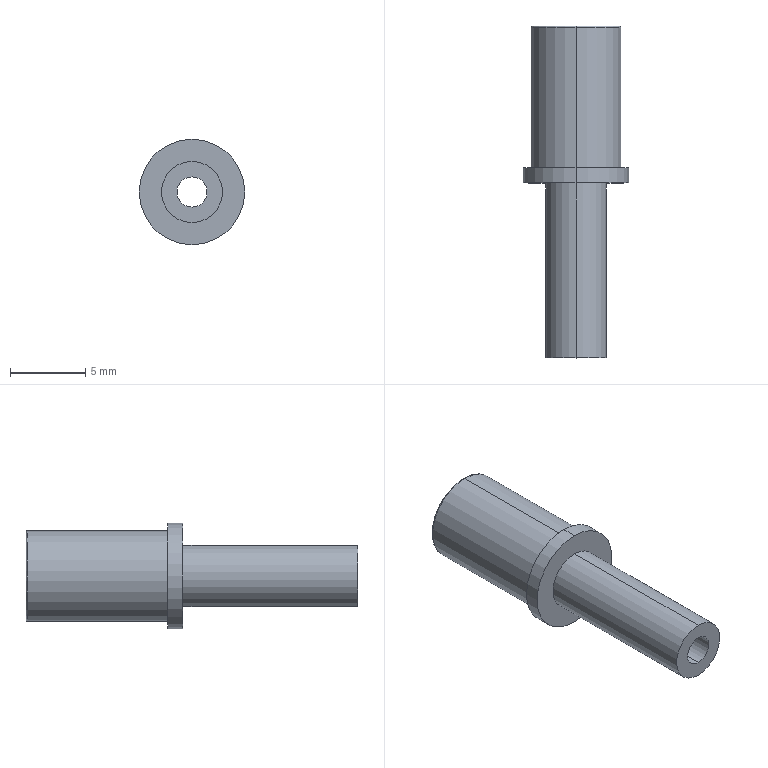Part | SolidWorks | features Fillet 1, Revolution 1 | 1 solid | 14 faces | box 7 x 22 x 7 mm | volume 384.292 mm3 | cylinder 8 | plane 4 | torus 2 | commonest cylinder face diameters 2 x2 4.047 x2 6 x2 7 x2
STEP:
#1=CARTESIAN_POINT('',(0.,10.4,2.9));
#2=VERTEX_POINT('',#1);
#3=CARTESIAN_POINT('',(0.,10.4,-2.9));
#4=VERTEX_POINT('',#3);
#5=CARTESIAN_POINT('',(0.,10.4,0.));
#6=DIRECTION('',(0.,1.,0.));
#7=DIRECTION('',(0.,0.,-1.));
#8=AXIS2_PLACEMENT_3D('',#5,#6,#7);
#9=CIRCLE('',#8,2.9);
#10=EDGE_CURVE('',#2,#4,#9,.T.);
#11=ORIENTED_EDGE('',*,*,#10,.F.);
#12=CARTESIAN_POINT('',(0.,10.3,3.));
#13=VERTEX_POINT('',#12);
#14=CARTESIAN_POINT('',(0.,10.3,2.9));
#15=DIRECTION('',(1.,0.,0.));
#16=DIRECTION('',(0.,0.,-1.));
#17=AXIS2_PLACEMENT_3D('',#14,#15,#16);
#18=CIRCLE('',#17,0.1);
#19=EDGE_CURVE('',#2,#13,#18,.T.);
#20=ORIENTED_EDGE('',*,*,#19,.T.);
#21=CARTESIAN_POINT('',(0.,10.3,-3.));
#22=VERTEX_POINT('',#21);
#23=CARTESIAN_POINT('',(0.,10.3,0.));
#24=DIRECTION('',(0.,-1.,0.));
#25=DIRECTION('',(0.,0.,-1.));
#26=AXIS2_PLACEMENT_3D('',#23,#24,#25);
#27=CIRCLE('',#26,3.);
#28=EDGE_CURVE('',#22,#13,#27,.T.);
#29=ORIENTED_EDGE('',*,*,#28,.F.);
#30=CARTESIAN_POINT('',(0.,10.3,-2.9));
#31=DIRECTION('',(-1.,0.,0.));
#32=DIRECTION('',(0.,0.,1.));
#33=AXIS2_PLACEMENT_3D('',#30,#31,#32);
#34=CIRCLE('',#33,0.1);
#35=EDGE_CURVE('',#4,#22,#34,.T.);
#36=ORIENTED_EDGE('',*,*,#35,.F.);
#37=EDGE_LOOP('',(#11,#20,#29,#36));
#38=FACE_OUTER_BOUND('',#37,.T.);
#39=CARTESIAN_POINT('',(0.,10.3,0.));
#40=DIRECTION('',(0.,-1.,0.));
#41=DIRECTION('',(0.,0.,-1.));
#42=AXIS2_PLACEMENT_3D('',#39,#40,#41);
#43=TOROIDAL_SURFACE('',#42,2.9,0.1);
#44=ADVANCED_FACE('',(#38),#43,.T.);
#45=CARTESIAN_POINT('',(0.,1.,-3.5));
#46=VERTEX_POINT('',#45);
#47=CARTESIAN_POINT('',(0.,1.,3.5));
#48=VERTEX_POINT('',#47);
#49=CARTESIAN_POINT('',(0.,1.,0.));
#50=DIRECTION('',(0.,-1.,0.));
#51=DIRECTION('',(0.,0.,-1.));
#52=AXIS2_PLACEMENT_3D('',#49,#50,#51);
#53=CIRCLE('',#52,3.5);
#54=EDGE_CURVE('',#46,#48,#53,.T.);
#55=ORIENTED_EDGE('',*,*,#54,.T.);
#56=CARTESIAN_POINT('',(0.,0.,3.5));
#57=VERTEX_POINT('',#56);
#58=CARTESIAN_POINT('',(0.,-19.747,3.5));
#59=DIRECTION('',(0.,-1.,0.));
#60=VECTOR('',#59,1000.);
#61=LINE('',#58,#60);
#62=EDGE_CURVE('',#48,#57,#61,.T.);
#63=ORIENTED_EDGE('',*,*,#62,.T.);
#64=CARTESIAN_POINT('',(0.,0.,-3.5));
#65=VERTEX_POINT('',#64);
#66=CARTESIAN_POINT('',(0.,0.,0.));
#67=DIRECTION('',(0.,-1.,0.));
#68=DIRECTION('',(0.,0.,-1.));
#69=AXIS2_PLACEMENT_3D('',#66,#67,#68);
#70=CIRCLE('',#69,3.5);
#71=EDGE_CURVE('',#65,#57,#70,.T.);
#72=ORIENTED_EDGE('',*,*,#71,.F.);
#73=CARTESIAN_POINT('',(0.,-19.747,-3.5));
#74=DIRECTION('',(0.,-1.,0.));
#75=VECTOR('',#74,1000.);
#76=LINE('',#73,#75);
#77=EDGE_CURVE('',#46,#65,#76,.T.);
#78=ORIENTED_EDGE('',*,*,#77,.F.);
#79=EDGE_LOOP('',(#55,#63,#72,#78));
#80=FACE_OUTER_BOUND('',#79,.T.);
#81=CARTESIAN_POINT('',(0.,-19.747,0.));
#82=DIRECTION('',(0.,-1.,0.));
#83=DIRECTION('',(0.,0.,-1.));
#84=AXIS2_PLACEMENT_3D('',#81,#82,#83);
#85=CYLINDRICAL_SURFACE('',#84,3.5);
#86=ADVANCED_FACE('',(#80),#85,.T.);
#87=CARTESIAN_POINT('',(0.,0.,-2.023));
#88=VERTEX_POINT('',#87);
#89=CARTESIAN_POINT('',(0.,0.,2.023));
#90=VERTEX_POINT('',#89);
#91=CARTESIAN_POINT('',(0.,0.,0.));
#92=DIRECTION('',(0.,-1.,0.));
#93=DIRECTION('',(0.,0.,-1.));
#94=AXIS2_PLACEMENT_3D('',#91,#92,#93);
#95=CIRCLE('',#94,2.023);
#96=EDGE_CURVE('',#88,#90,#95,.T.);
#97=ORIENTED_EDGE('',*,*,#96,.T.);
#98=CARTESIAN_POINT('',(0.,-11.6,2.023));
#99=VERTEX_POINT('',#98);
#100=CARTESIAN_POINT('',(0.,-19.747,2.023));
#101=DIRECTION('',(0.,-1.,0.));
#102=VECTOR('',#101,1000.);
#103=LINE('',#100,#102);
#104=EDGE_CURVE('',#90,#99,#103,.T.);
#105=ORIENTED_EDGE('',*,*,#104,.T.);
#106=CARTESIAN_POINT('',(0.,-11.6,-2.023));
#107=VERTEX_POINT('',#106);
#108=CARTESIAN_POINT('',(0.,-11.6,0.));
#109=DIRECTION('',(0.,-1.,0.));
#110=DIRECTION('',(0.,0.,-1.));
#111=AXIS2_PLACEMENT_3D('',#108,#109,#110);
#112=CIRCLE('',#111,2.023);
#113=EDGE_CURVE('',#107,#99,#112,.T.);
#114=ORIENTED_EDGE('',*,*,#113,.F.);
#115=CARTESIAN_POINT('',(0.,-19.747,-2.023));
#116=DIRECTION('',(0.,-1.,0.));
#117=VECTOR('',#116,1000.);
#118=LINE('',#115,#117);
#119=EDGE_CURVE('',#88,#107,#118,.T.);
#120=ORIENTED_EDGE('',*,*,#119,.F.);
#121=EDGE_LOOP('',(#97,#105,#114,#120));
#122=FACE_OUTER_BOUND('',#121,.T.);
#123=CARTESIAN_POINT('',(0.,-19.747,0.));
#124=DIRECTION('',(0.,-1.,0.));
#125=DIRECTION('',(0.,0.,-1.));
#126=AXIS2_PLACEMENT_3D('',#123,#124,#125);
#127=CYLINDRICAL_SURFACE('',#126,2.023);
#128=ADVANCED_FACE('',(#122),#127,.T.);
#129=CARTESIAN_POINT('',(0.,10.4,1.));
#130=VERTEX_POINT('',#129);
#131=CARTESIAN_POINT('',(0.,10.4,-1.));
#132=VERTEX_POINT('',#131);
#133=CARTESIAN_POINT('',(0.,10.4,0.));
#134=DIRECTION('',(0.,-1.,0.));
#135=DIRECTION('',(0.,0.,-1.));
#136=AXIS2_PLACEMENT_3D('',#133,#134,#135);
#137=CIRCLE('',#136,1.);
#138=EDGE_CURVE('',#130,#132,#137,.T.);
#139=ORIENTED_EDGE('',*,*,#138,.F.);
#140=CARTESIAN_POINT('',(0.,-11.6,1.));
#141=VERTEX_POINT('',#140);
#142=CARTESIAN_POINT('',(0.,-19.747,1.));
#143=DIRECTION('',(0.,-1.,0.));
#144=VECTOR('',#143,1000.);
#145=LINE('',#142,#144);
#146=EDGE_CURVE('',#130,#141,#145,.T.);
#147=ORIENTED_EDGE('',*,*,#146,.T.);
#148=CARTESIAN_POINT('',(0.,-11.6,-1.));
#149=VERTEX_POINT('',#148);
#150=CARTESIAN_POINT('',(0.,-11.6,0.));
#151=DIRECTION('',(0.,-1.,0.));
#152=DIRECTION('',(0.,0.,-1.));
#153=AXIS2_PLACEMENT_3D('',#150,#151,#152);
#154=CIRCLE('',#153,1.);
#155=EDGE_CURVE('',#141,#149,#154,.T.);
#156=ORIENTED_EDGE('',*,*,#155,.T.);
#157=CARTESIAN_POINT('',(0.,-19.747,-1.));
#158=DIRECTION('',(0.,-1.,0.));
#159=VECTOR('',#158,1000.);
#160=LINE('',#157,#159);
#161=EDGE_CURVE('',#132,#149,#160,.T.);
#162=ORIENTED_EDGE('',*,*,#161,.F.);
#163=EDGE_LOOP('',(#139,#147,#156,#162));
#164=FACE_OUTER_BOUND('',#163,.T.);
#165=CARTESIAN_POINT('',(0.,-19.747,0.));
#166=DIRECTION('',(0.,-1.,0.));
#167=DIRECTION('',(0.,0.,-1.));
#168=AXIS2_PLACEMENT_3D('',#165,#166,#167);
#169=CYLINDRICAL_SURFACE('',#168,1.);
#170=ADVANCED_FACE('',(#164),#169,.F.);
#171=ORIENTED_EDGE('',*,*,#28,.T.);
#172=CARTESIAN_POINT('',(0.,1.,3.));
#173=VERTEX_POINT('',#172);
#174=CARTESIAN_POINT('',(0.,-19.747,3.));
#175=DIRECTION('',(0.,-1.,0.));
#176=VECTOR('',#175,1000.);
#177=LINE('',#174,#176);
#178=EDGE_CURVE('',#13,#173,#177,.T.);
#179=ORIENTED_EDGE('',*,*,#178,.T.);
#180=CARTESIAN_POINT('',(0.,1.,-3.));
#181=VERTEX_POINT('',#180);
#182=CARTESIAN_POINT('',(0.,1.,0.));
#183=DIRECTION('',(0.,-1.,0.));
#184=DIRECTION('',(0.,0.,-1.));
#185=AXIS2_PLACEMENT_3D('',#182,#183,#184);
#186=CIRCLE('',#185,3.);
#187=EDGE_CURVE('',#181,#173,#186,.T.);
#188=ORIENTED_EDGE('',*,*,#187,.F.);
#189=CARTESIAN_POINT('',(0.,-19.747,-3.));
#190=DIRECTION('',(0.,-1.,0.));
#191=VECTOR('',#190,1000.);
#192=LINE('',#189,#191);
#193=EDGE_CURVE('',#22,#181,#192,.T.);
#194=ORIENTED_EDGE('',*,*,#193,.F.);
#195=EDGE_LOOP('',(#171,#179,#188,#194));
#196=FACE_OUTER_BOUND('',#195,.T.);
#197=CARTESIAN_POINT('',(0.,-19.747,0.));
#198=DIRECTION('',(0.,-1.,0.));
#199=DIRECTION('',(0.,0.,-1.));
#200=AXIS2_PLACEMENT_3D('',#197,#198,#199);
#201=CYLINDRICAL_SURFACE('',#200,3.);
#202=ADVANCED_FACE('',(#196),#201,.T.);
#203=ORIENTED_EDGE('',*,*,#178,.F.);
#204=CARTESIAN_POINT('',(0.,10.3,0.));
#205=DIRECTION('',(0.,-1.,0.));
#206=DIRECTION('',(0.,0.,-1.));
#207=AXIS2_PLACEMENT_3D('',#204,#205,#206);
#208=CIRCLE('',#207,3.);
#209=EDGE_CURVE('',#13,#22,#208,.T.);
#210=ORIENTED_EDGE('',*,*,#209,.T.);
#211=ORIENTED_EDGE('',*,*,#193,.T.);
#212=CARTESIAN_POINT('',(0.,1.,0.));
#213=DIRECTION('',(0.,-1.,0.));
#214=DIRECTION('',(0.,0.,-1.));
#215=AXIS2_PLACEMENT_3D('',#212,#213,#214);
#216=CIRCLE('',#215,3.);
#217=EDGE_CURVE('',#173,#181,#216,.T.);
#218=ORIENTED_EDGE('',*,*,#217,.F.);
#219=EDGE_LOOP('',(#203,#210,#211,#218));
#220=FACE_OUTER_BOUND('',#219,.T.);
#221=CARTESIAN_POINT('',(0.,-19.747,0.));
#222=DIRECTION('',(0.,-1.,0.));
#223=DIRECTION('',(0.,0.,-1.));
#224=AXIS2_PLACEMENT_3D('',#221,#222,#223);
#225=CYLINDRICAL_SURFACE('',#224,3.);
#226=ADVANCED_FACE('',(#220),#225,.T.);
#227=CARTESIAN_POINT('',(0.,10.4,0.));
#228=DIRECTION('',(0.,1.,0.));
#229=DIRECTION('',(0.,0.,-1.));
#230=AXIS2_PLACEMENT_3D('',#227,#228,#229);
#231=CIRCLE('',#230,2.9);
#232=EDGE_CURVE('',#4,#2,#231,.T.);
#233=ORIENTED_EDGE('',*,*,#232,.T.);
#234=ORIENTED_EDGE('',*,*,#10,.T.);
#235=EDGE_LOOP('',(#233,#234));
#236=FACE_OUTER_BOUND('',#235,.T.);
#237=CARTESIAN_POINT('',(0.,10.4,0.));
#238=DIRECTION('',(0.,-1.,0.));
#239=DIRECTION('',(0.,0.,-1.));
#240=AXIS2_PLACEMENT_3D('',#237,#238,#239);
#241=CIRCLE('',#240,1.);
#242=EDGE_CURVE('',#132,#130,#241,.T.);
#243=ORIENTED_EDGE('',*,*,#242,.T.);
#244=ORIENTED_EDGE('',*,*,#138,.T.);
#245=EDGE_LOOP('',(#243,#244));
#246=FACE_BOUND('',#245,.T.);
#247=CARTESIAN_POINT('',(-3.,10.4,0.));
#248=DIRECTION('',(0.,-1.,0.));
#249=DIRECTION('',(0.,0.,-1.));
#250=AXIS2_PLACEMENT_3D('',#247,#248,#249);
#251=PLANE('',#250);
#252=ADVANCED_FACE('',(#236,#246),#251,.F.);
#253=ORIENTED_EDGE('',*,*,#146,.F.);
#254=ORIENTED_EDGE('',*,*,#242,.F.);
#255=ORIENTED_EDGE('',*,*,#161,.T.);
#256=CARTESIAN_POINT('',(0.,-11.6,0.));
#257=DIRECTION('',(0.,-1.,0.));
#258=DIRECTION('',(0.,0.,-1.));
#259=AXIS2_PLACEMENT_3D('',#256,#257,#258);
#260=CIRCLE('',#259,1.);
#261=EDGE_CURVE('',#149,#141,#260,.T.);
#262=ORIENTED_EDGE('',*,*,#261,.T.);
#263=EDGE_LOOP('',(#253,#254,#255,#262));
#264=FACE_OUTER_BOUND('',#263,.T.);
#265=CARTESIAN_POINT('',(0.,-19.747,0.));
#266=DIRECTION('',(0.,-1.,0.));
#267=DIRECTION('',(0.,0.,-1.));
#268=AXIS2_PLACEMENT_3D('',#265,#266,#267);
#269=CYLINDRICAL_SURFACE('',#268,1.);
#270=ADVANCED_FACE('',(#264),#269,.F.);
#271=ORIENTED_EDGE('',*,*,#261,.F.);
#272=ORIENTED_EDGE('',*,*,#155,.F.);
#273=EDGE_LOOP('',(#271,#272));
#274=FACE_BOUND('',#273,.T.);
#275=ORIENTED_EDGE('',*,*,#113,.T.);
#276=CARTESIAN_POINT('',(0.,-11.6,0.));
#277=DIRECTION('',(0.,-1.,0.));
#278=DIRECTION('',(0.,0.,-1.));
#279=AXIS2_PLACEMENT_3D('',#276,#277,#278);
#280=CIRCLE('',#279,2.023);
#281=EDGE_CURVE('',#99,#107,#280,.T.);
#282=ORIENTED_EDGE('',*,*,#281,.T.);
#283=EDGE_LOOP('',(#275,#282));
#284=FACE_OUTER_BOUND('',#283,.T.);
#285=CARTESIAN_POINT('',(-1.,-11.6,0.));
#286=DIRECTION('',(0.,1.,0.));
#287=DIRECTION('',(0.,0.,1.));
#288=AXIS2_PLACEMENT_3D('',#285,#286,#287);
#289=PLANE('',#288);
#290=ADVANCED_FACE('',(#274,#284),#289,.F.);
#291=ORIENTED_EDGE('',*,*,#104,.F.);
#292=CARTESIAN_POINT('',(0.,0.,0.));
#293=DIRECTION('',(0.,-1.,0.));
#294=DIRECTION('',(0.,0.,-1.));
#295=AXIS2_PLACEMENT_3D('',#292,#293,#294);
#296=CIRCLE('',#295,2.023);
#297=EDGE_CURVE('',#90,#88,#296,.T.);
#298=ORIENTED_EDGE('',*,*,#297,.T.);
#299=ORIENTED_EDGE('',*,*,#119,.T.);
#300=ORIENTED_EDGE('',*,*,#281,.F.);
#301=EDGE_LOOP('',(#291,#298,#299,#300));
#302=FACE_OUTER_BOUND('',#301,.T.);
#303=CARTESIAN_POINT('',(0.,-19.747,0.));
#304=DIRECTION('',(0.,-1.,0.));
#305=DIRECTION('',(0.,0.,-1.));
#306=AXIS2_PLACEMENT_3D('',#303,#304,#305);
#307=CYLINDRICAL_SURFACE('',#306,2.023);
#308=ADVANCED_FACE('',(#302),#307,.T.);
#309=ORIENTED_EDGE('',*,*,#96,.F.);
#310=ORIENTED_EDGE('',*,*,#297,.F.);
#311=EDGE_LOOP('',(#309,#310));
#312=FACE_BOUND('',#311,.T.);
#313=ORIENTED_EDGE('',*,*,#71,.T.);
#314=CARTESIAN_POINT('',(0.,0.,0.));
#315=DIRECTION('',(0.,-1.,0.));
#316=DIRECTION('',(0.,0.,-1.));
#317=AXIS2_PLACEMENT_3D('',#314,#315,#316);
#318=CIRCLE('',#317,3.5);
#319=EDGE_CURVE('',#57,#65,#318,.T.);
#320=ORIENTED_EDGE('',*,*,#319,.T.);
#321=EDGE_LOOP('',(#313,#320));
#322=FACE_OUTER_BOUND('',#321,.T.);
#323=CARTESIAN_POINT('',(-3.5,0.,0.));
#324=DIRECTION('',(0.,1.,0.));
#325=DIRECTION('',(0.,0.,1.));
#326=AXIS2_PLACEMENT_3D('',#323,#324,#325);
#327=PLANE('',#326);
#328=ADVANCED_FACE('',(#312,#322),#327,.F.);
#329=ORIENTED_EDGE('',*,*,#62,.F.);
#330=CARTESIAN_POINT('',(0.,1.,0.));
#331=DIRECTION('',(0.,-1.,0.));
#332=DIRECTION('',(0.,0.,-1.));
#333=AXIS2_PLACEMENT_3D('',#330,#331,#332);
#334=CIRCLE('',#333,3.5);
#335=EDGE_CURVE('',#48,#46,#334,.T.);
#336=ORIENTED_EDGE('',*,*,#335,.T.);
#337=ORIENTED_EDGE('',*,*,#77,.T.);
#338=ORIENTED_EDGE('',*,*,#319,.F.);
#339=EDGE_LOOP('',(#329,#336,#337,#338));
#340=FACE_OUTER_BOUND('',#339,.T.);
#341=CARTESIAN_POINT('',(0.,-19.747,0.));
#342=DIRECTION('',(0.,-1.,0.));
#343=DIRECTION('',(0.,0.,-1.));
#344=AXIS2_PLACEMENT_3D('',#341,#342,#343);
#345=CYLINDRICAL_SURFACE('',#344,3.5);
#346=ADVANCED_FACE('',(#340),#345,.T.);
#347=ORIENTED_EDGE('',*,*,#54,.F.);
#348=ORIENTED_EDGE('',*,*,#335,.F.);
#349=EDGE_LOOP('',(#347,#348));
#350=FACE_OUTER_BOUND('',#349,.T.);
#351=ORIENTED_EDGE('',*,*,#187,.T.);
#352=ORIENTED_EDGE('',*,*,#217,.T.);
#353=EDGE_LOOP('',(#351,#352));
#354=FACE_BOUND('',#353,.T.);
#355=CARTESIAN_POINT('',(-3.5,1.,0.));
#356=DIRECTION('',(0.,-1.,0.));
#357=DIRECTION('',(0.,0.,-1.));
#358=AXIS2_PLACEMENT_3D('',#355,#356,#357);
#359=PLANE('',#358);
#360=ADVANCED_FACE('',(#350,#354),#359,.F.);
#361=ORIENTED_EDGE('',*,*,#19,.F.);
#362=ORIENTED_EDGE('',*,*,#232,.F.);
#363=ORIENTED_EDGE('',*,*,#35,.T.);
#364=ORIENTED_EDGE('',*,*,#209,.F.);
#365=EDGE_LOOP('',(#361,#362,#363,#364));
#366=FACE_OUTER_BOUND('',#365,.T.);
#367=CARTESIAN_POINT('',(0.,10.3,0.));
#368=DIRECTION('',(0.,-1.,0.));
#369=DIRECTION('',(0.,0.,-1.));
#370=AXIS2_PLACEMENT_3D('',#367,#368,#369);
#371=TOROIDAL_SURFACE('',#370,2.9,0.1);
#372=ADVANCED_FACE('',(#366),#371,.T.);
#373=CLOSED_SHELL('',(#44,#86,#128,#170,#202,#226,#252,#270,#290,#308,#328,#346,#360,#372));
#374=MANIFOLD_SOLID_BREP('',#373);
#375=CARTESIAN_POINT('',(0.,0.,0.));
#376=DIRECTION('',(0.,0.,1.));
#377=DIRECTION('',(1.,0.,0.));
#378=AXIS2_PLACEMENT_3D('',#375,#376,#377);
#379=(LENGTH_UNIT()NAMED_UNIT(*)SI_UNIT(.MILLI.,.METRE.));
#380=UNCERTAINTY_MEASURE_WITH_UNIT(LENGTH_MEASURE(0.00001),#379,'','');
#381=(NAMED_UNIT(*)PLANE_ANGLE_UNIT()SI_UNIT($,.RADIAN.));
#382=(NAMED_UNIT(*)SI_UNIT($,.STERADIAN.)SOLID_ANGLE_UNIT());
#383=(GEOMETRIC_REPRESENTATION_CONTEXT(3)GLOBAL_UNCERTAINTY_ASSIGNED_CONTEXT((#380))GLOBAL_UNIT_ASSIGNED_CONTEXT((#379,#381,#382))REPRESENTATION_CONTEXT('',''));
#384=ADVANCED_BREP_SHAPE_REPRESENTATION('',(#374,#378),#383);